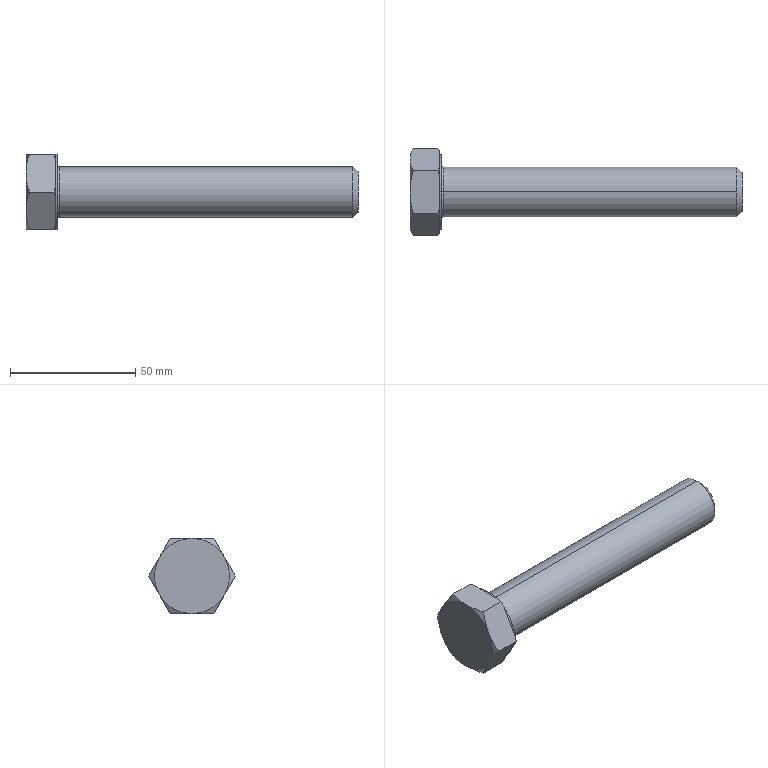Part | STEP file | GB/T 5780-2000 hex head bolt, grade C, M20×120 (3.6 grade) | 1 solid | 35 faces | box 132.5 x 34.641 x 30 mm | volume 47244 mm3 | plane 15 | cone 14 | cylinder 4 | torus 2 | commonest cylinder face diameters 20 x2 30 x2